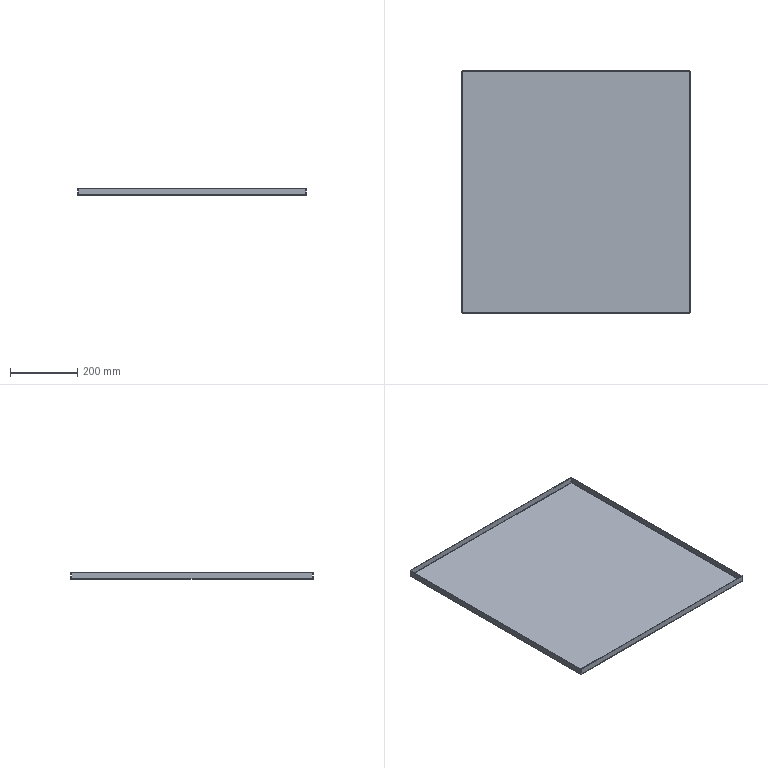Part | STEP file | Part 8 | 1 solid | 38 faces | box 680 x 720 x 20 mm | volume 1075588 mm3 | plane 22 | spline 8 | cylinder 8 | commonest cylinder face diameters 1 x4 5 x4
STEP:
#1=CARTESIAN_POINT('',(-337.5,-357.5,-2.));
#2=VERTEX_POINT('',#1);
#3=CARTESIAN_POINT('',(-337.5,357.5,-2.));
#4=VERTEX_POINT('',#3);
#5=CARTESIAN_POINT('',(-337.5,-357.5,-2.));
#6=DIRECTION('',(0.,1.,0.));
#7=VECTOR('',#6,1000.);
#8=LINE('',#5,#7);
#9=EDGE_CURVE('',#2,#4,#8,.T.);
#10=ORIENTED_EDGE('',*,*,#9,.T.);
#11=CARTESIAN_POINT('',(337.5,357.5,-2.));
#12=VERTEX_POINT('',#11);
#13=CARTESIAN_POINT('',(-337.5,357.5,-2.));
#14=DIRECTION('',(1.,0.,0.));
#15=VECTOR('',#14,1000.);
#16=LINE('',#13,#15);
#17=EDGE_CURVE('',#4,#12,#16,.T.);
#18=ORIENTED_EDGE('',*,*,#17,.T.);
#19=CARTESIAN_POINT('',(337.5,-357.5,-2.));
#20=VERTEX_POINT('',#19);
#21=CARTESIAN_POINT('',(337.5,357.5,-2.));
#22=DIRECTION('',(0.,-1.,0.));
#23=VECTOR('',#22,1000.);
#24=LINE('',#21,#23);
#25=EDGE_CURVE('',#12,#20,#24,.T.);
#26=ORIENTED_EDGE('',*,*,#25,.T.);
#27=CARTESIAN_POINT('',(337.5,-357.5,-2.));
#28=DIRECTION('',(-1.,0.,0.));
#29=VECTOR('',#28,1000.);
#30=LINE('',#27,#29);
#31=EDGE_CURVE('',#20,#2,#30,.T.);
#32=ORIENTED_EDGE('',*,*,#31,.T.);
#33=EDGE_LOOP('',(#10,#18,#26,#32));
#34=FACE_OUTER_BOUND('',#33,.T.);
#35=CARTESIAN_POINT('',(0.,0.,-2.));
#36=DIRECTION('',(0.,0.,1.));
#37=DIRECTION('',(1.,0.,0.));
#38=AXIS2_PLACEMENT_3D('',#35,#36,#37);
#39=PLANE('',#38);
#40=ADVANCED_FACE('',(#34),#39,.F.);
#41=CARTESIAN_POINT('',(-337.5,357.5,0.));
#42=VERTEX_POINT('',#41);
#43=CARTESIAN_POINT('',(337.5,357.5,0.));
#44=VERTEX_POINT('',#43);
#45=CARTESIAN_POINT('',(-337.5,357.5,0.));
#46=DIRECTION('',(1.,0.,0.));
#47=VECTOR('',#46,1000.);
#48=LINE('',#45,#47);
#49=EDGE_CURVE('',#42,#44,#48,.T.);
#50=ORIENTED_EDGE('',*,*,#49,.F.);
#51=CARTESIAN_POINT('',(-337.5,-357.5,0.));
#52=VERTEX_POINT('',#51);
#53=CARTESIAN_POINT('',(-337.5,-357.5,0.));
#54=DIRECTION('',(0.,1.,0.));
#55=VECTOR('',#54,1000.);
#56=LINE('',#53,#55);
#57=EDGE_CURVE('',#52,#42,#56,.T.);
#58=ORIENTED_EDGE('',*,*,#57,.F.);
#59=CARTESIAN_POINT('',(337.5,-357.5,0.));
#60=VERTEX_POINT('',#59);
#61=CARTESIAN_POINT('',(337.5,-357.5,0.));
#62=DIRECTION('',(-1.,0.,0.));
#63=VECTOR('',#62,1000.);
#64=LINE('',#61,#63);
#65=EDGE_CURVE('',#60,#52,#64,.T.);
#66=ORIENTED_EDGE('',*,*,#65,.F.);
#67=CARTESIAN_POINT('',(337.5,357.5,0.));
#68=DIRECTION('',(0.,-1.,0.));
#69=VECTOR('',#68,1000.);
#70=LINE('',#67,#69);
#71=EDGE_CURVE('',#44,#60,#70,.T.);
#72=ORIENTED_EDGE('',*,*,#71,.F.);
#73=EDGE_LOOP('',(#50,#58,#66,#72));
#74=FACE_OUTER_BOUND('',#73,.T.);
#75=CARTESIAN_POINT('',(0.,0.,0.));
#76=DIRECTION('',(0.,0.,1.));
#77=DIRECTION('',(1.,0.,0.));
#78=AXIS2_PLACEMENT_3D('',#75,#76,#77);
#79=PLANE('',#78);
#80=ADVANCED_FACE('',(#74),#79,.T.);
#81=CARTESIAN_POINT('',(337.293,360.,0.5));
#82=VERTEX_POINT('',#81);
#83=CARTESIAN_POINT('',(337.293,358.,0.5));
#84=VERTEX_POINT('',#83);
#85=CARTESIAN_POINT('',(337.293,358.,0.5));
#86=DIRECTION('',(0.,-1.,0.));
#87=VECTOR('',#86,1000.);
#88=LINE('',#85,#87);
#89=EDGE_CURVE('',#82,#84,#88,.T.);
#90=ORIENTED_EDGE('',*,*,#89,.T.);
#91=CARTESIAN_POINT('',(337.5,357.5,0.));
#92=CARTESIAN_POINT('',(337.465,357.631,0.));
#93=CARTESIAN_POINT('',(337.431,357.761,0.05389));
#94=CARTESIAN_POINT('',(337.362,357.946,0.239));
#95=CARTESIAN_POINT('',(337.327,358.,0.3691));
#96=CARTESIAN_POINT('',(337.293,358.,0.5));
#97=B_SPLINE_CURVE_WITH_KNOTS('',3,(#91,#92,#93,#94,#95,#96),.UNSPECIFIED.,.F.,.F.,(4,2,4),(0.,0.5,1.),.UNSPECIFIED.);
#98=EDGE_CURVE('',#44,#84,#97,.T.);
#99=ORIENTED_EDGE('',*,*,#98,.F.);
#100=CARTESIAN_POINT('',(337.5,357.5,0.));
#101=DIRECTION('',(0.,0.,-1.));
#102=VECTOR('',#101,1000.);
#103=LINE('',#100,#102);
#104=EDGE_CURVE('',#44,#12,#103,.T.);
#105=ORIENTED_EDGE('',*,*,#104,.T.);
#106=CARTESIAN_POINT('',(337.5,357.5,-2.));
#107=CARTESIAN_POINT('',(337.483,357.827,-2.));
#108=CARTESIAN_POINT('',(337.465,358.154,-1.935));
#109=CARTESIAN_POINT('',(337.431,358.759,-1.684));
#110=CARTESIAN_POINT('',(337.414,359.036,-1.499));
#111=CARTESIAN_POINT('',(337.379,359.499,-1.036));
#112=CARTESIAN_POINT('',(337.362,359.684,-0.759));
#113=CARTESIAN_POINT('',(337.327,359.935,-0.1544));
#114=CARTESIAN_POINT('',(337.31,360.,0.1728));
#115=CARTESIAN_POINT('',(337.293,360.,0.5));
#116=B_SPLINE_CURVE_WITH_KNOTS('',3,(#106,#107,#108,#109,#110,#111,#112,#113,#114,#115),.UNSPECIFIED.,.F.,.F.,(4,2,2,2,4),(0.,0.25,0.5,0.75,1.),.UNSPECIFIED.);
#117=EDGE_CURVE('',#12,#82,#116,.T.);
#118=ORIENTED_EDGE('',*,*,#117,.T.);
#119=EDGE_LOOP('',(#90,#99,#105,#118));
#120=FACE_OUTER_BOUND('',#119,.T.);
#121=CARTESIAN_POINT('',(337.5,357.5,-2.02));
#122=CARTESIAN_POINT('',(337.483,357.83,-2.02));
#123=CARTESIAN_POINT('',(337.465,358.16,-1.954));
#124=CARTESIAN_POINT('',(337.431,358.769,-1.702));
#125=CARTESIAN_POINT('',(337.414,359.049,-1.515));
#126=CARTESIAN_POINT('',(337.379,359.515,-1.049));
#127=CARTESIAN_POINT('',(337.362,359.702,-0.7691));
#128=CARTESIAN_POINT('',(337.327,359.954,-0.1596));
#129=CARTESIAN_POINT('',(337.31,360.02,0.1701));
#130=CARTESIAN_POINT('',(337.293,360.02,0.5));
#131=CARTESIAN_POINT('',(337.5,357.5,-2.));
#132=CARTESIAN_POINT('',(337.483,357.827,-2.));
#133=CARTESIAN_POINT('',(337.465,358.154,-1.935));
#134=CARTESIAN_POINT('',(337.431,358.759,-1.684));
#135=CARTESIAN_POINT('',(337.414,359.036,-1.499));
#136=CARTESIAN_POINT('',(337.379,359.499,-1.036));
#137=CARTESIAN_POINT('',(337.362,359.684,-0.759));
#138=CARTESIAN_POINT('',(337.327,359.935,-0.1544));
#139=CARTESIAN_POINT('',(337.31,360.,0.1727));
#140=CARTESIAN_POINT('',(337.293,360.,0.5));
#141=CARTESIAN_POINT('',(337.5,357.5,0.));
#142=CARTESIAN_POINT('',(337.483,357.565,0.));
#143=CARTESIAN_POINT('',(337.465,357.631,0.01301));
#144=CARTESIAN_POINT('',(337.431,357.752,0.06311));
#145=CARTESIAN_POINT('',(337.414,357.807,0.1002));
#146=CARTESIAN_POINT('',(337.379,357.9,0.1927));
#147=CARTESIAN_POINT('',(337.362,357.937,0.2482));
#148=CARTESIAN_POINT('',(337.327,357.987,0.3691));
#149=CARTESIAN_POINT('',(337.31,358.,0.4345));
#150=CARTESIAN_POINT('',(337.293,358.,0.5));
#151=CARTESIAN_POINT('',(337.5,357.5,0.0202));
#152=CARTESIAN_POINT('',(337.483,357.563,0.0202));
#153=CARTESIAN_POINT('',(337.465,357.626,0.03269));
#154=CARTESIAN_POINT('',(337.431,357.742,0.08076));
#155=CARTESIAN_POINT('',(337.414,357.795,0.1163));
#156=CARTESIAN_POINT('',(337.379,357.884,0.2051));
#157=CARTESIAN_POINT('',(337.362,357.919,0.2584));
#158=CARTESIAN_POINT('',(337.327,357.967,0.3744));
#159=CARTESIAN_POINT('',(337.31,357.98,0.4372));
#160=CARTESIAN_POINT('',(337.293,357.98,0.5));
#161=B_SPLINE_SURFACE_WITH_KNOTS('',1,3,((#121,#122,#123,#124,#125,#126,#127,#128,#129,#130),(#131,#132,#133,#134,#135,#136,#137,#138,#139,#140),(#141,#142,#143,#144,#145,#146,#147,#148,#149,#150),(#151,#152,#153,#154,#155,#156,#157,#158,#159,#160)),.UNSPECIFIED.,.F.,.F.,.F.,(2,1,1,2),(4,2,2,2,4),(-0.01,0.,1.,1.01),(0.,0.25,0.5,0.75,1.),.UNSPECIFIED.);
#162=ADVANCED_FACE('',(#120),#161,.F.);
#163=CARTESIAN_POINT('',(-337.293,358.,0.5));
#164=VERTEX_POINT('',#163);
#165=CARTESIAN_POINT('',(-337.293,358.,0.5));
#166=CARTESIAN_POINT('',(-337.327,358.,0.3691));
#167=CARTESIAN_POINT('',(-337.362,357.946,0.239));
#168=CARTESIAN_POINT('',(-337.431,357.761,0.05389));
#169=CARTESIAN_POINT('',(-337.465,357.631,0.));
#170=CARTESIAN_POINT('',(-337.5,357.5,0.));
#171=B_SPLINE_CURVE_WITH_KNOTS('',3,(#165,#166,#167,#168,#169,#170),.UNSPECIFIED.,.F.,.F.,(4,2,4),(0.,0.5,1.),.UNSPECIFIED.);
#172=EDGE_CURVE('',#164,#42,#171,.T.);
#173=ORIENTED_EDGE('',*,*,#172,.F.);
#174=CARTESIAN_POINT('',(-337.293,360.,0.5));
#175=VERTEX_POINT('',#174);
#176=CARTESIAN_POINT('',(-337.293,358.,0.5));
#177=DIRECTION('',(0.,-1.,0.));
#178=VECTOR('',#177,1000.);
#179=LINE('',#176,#178);
#180=EDGE_CURVE('',#175,#164,#179,.T.);
#181=ORIENTED_EDGE('',*,*,#180,.F.);
#182=CARTESIAN_POINT('',(-337.293,360.,0.5));
#183=CARTESIAN_POINT('',(-337.31,360.,0.1728));
#184=CARTESIAN_POINT('',(-337.327,359.935,-0.1544));
#185=CARTESIAN_POINT('',(-337.362,359.684,-0.759));
#186=CARTESIAN_POINT('',(-337.379,359.499,-1.036));
#187=CARTESIAN_POINT('',(-337.414,359.036,-1.499));
#188=CARTESIAN_POINT('',(-337.431,358.759,-1.684));
#189=CARTESIAN_POINT('',(-337.465,358.154,-1.935));
#190=CARTESIAN_POINT('',(-337.483,357.827,-2.));
#191=CARTESIAN_POINT('',(-337.5,357.5,-2.));
#192=B_SPLINE_CURVE_WITH_KNOTS('',3,(#182,#183,#184,#185,#186,#187,#188,#189,#190,#191),.UNSPECIFIED.,.F.,.F.,(4,2,2,2,4),(0.,0.25,0.5,0.75,1.),.UNSPECIFIED.);
#193=EDGE_CURVE('',#175,#4,#192,.T.);
#194=ORIENTED_EDGE('',*,*,#193,.T.);
#195=CARTESIAN_POINT('',(-337.5,357.5,0.));
#196=DIRECTION('',(0.,0.,-1.));
#197=VECTOR('',#196,1000.);
#198=LINE('',#195,#197);
#199=EDGE_CURVE('',#42,#4,#198,.T.);
#200=ORIENTED_EDGE('',*,*,#199,.F.);
#201=EDGE_LOOP('',(#173,#181,#194,#200));
#202=FACE_OUTER_BOUND('',#201,.T.);
#203=CARTESIAN_POINT('',(-337.293,360.02,0.5));
#204=CARTESIAN_POINT('',(-337.31,360.02,0.1701));
#205=CARTESIAN_POINT('',(-337.327,359.954,-0.1596));
#206=CARTESIAN_POINT('',(-337.362,359.702,-0.7691));
#207=CARTESIAN_POINT('',(-337.379,359.515,-1.049));
#208=CARTESIAN_POINT('',(-337.414,359.049,-1.515));
#209=CARTESIAN_POINT('',(-337.431,358.769,-1.702));
#210=CARTESIAN_POINT('',(-337.465,358.16,-1.954));
#211=CARTESIAN_POINT('',(-337.483,357.83,-2.02));
#212=CARTESIAN_POINT('',(-337.5,357.5,-2.02));
#213=CARTESIAN_POINT('',(-337.293,360.,0.5));
#214=CARTESIAN_POINT('',(-337.31,360.,0.1727));
#215=CARTESIAN_POINT('',(-337.327,359.935,-0.1544));
#216=CARTESIAN_POINT('',(-337.362,359.684,-0.759));
#217=CARTESIAN_POINT('',(-337.379,359.499,-1.036));
#218=CARTESIAN_POINT('',(-337.414,359.036,-1.499));
#219=CARTESIAN_POINT('',(-337.431,358.759,-1.684));
#220=CARTESIAN_POINT('',(-337.465,358.154,-1.935));
#221=CARTESIAN_POINT('',(-337.483,357.827,-2.));
#222=CARTESIAN_POINT('',(-337.5,357.5,-2.));
#223=CARTESIAN_POINT('',(-337.293,358.,0.5));
#224=CARTESIAN_POINT('',(-337.31,358.,0.4345));
#225=CARTESIAN_POINT('',(-337.327,357.987,0.3691));
#226=CARTESIAN_POINT('',(-337.362,357.937,0.2482));
#227=CARTESIAN_POINT('',(-337.379,357.9,0.1927));
#228=CARTESIAN_POINT('',(-337.414,357.807,0.1002));
#229=CARTESIAN_POINT('',(-337.431,357.752,0.06311));
#230=CARTESIAN_POINT('',(-337.465,357.631,0.01301));
#231=CARTESIAN_POINT('',(-337.483,357.565,0.));
#232=CARTESIAN_POINT('',(-337.5,357.5,0.));
#233=CARTESIAN_POINT('',(-337.293,357.98,0.5));
#234=CARTESIAN_POINT('',(-337.31,357.98,0.4372));
#235=CARTESIAN_POINT('',(-337.327,357.967,0.3744));
#236=CARTESIAN_POINT('',(-337.362,357.919,0.2584));
#237=CARTESIAN_POINT('',(-337.379,357.884,0.2051));
#238=CARTESIAN_POINT('',(-337.414,357.795,0.1163));
#239=CARTESIAN_POINT('',(-337.431,357.742,0.08076));
#240=CARTESIAN_POINT('',(-337.465,357.626,0.03269));
#241=CARTESIAN_POINT('',(-337.483,357.563,0.0202));
#242=CARTESIAN_POINT('',(-337.5,357.5,0.0202));
#243=B_SPLINE_SURFACE_WITH_KNOTS('',1,3,((#203,#204,#205,#206,#207,#208,#209,#210,#211,#212),(#213,#214,#215,#216,#217,#218,#219,#220,#221,#222),(#223,#224,#225,#226,#227,#228,#229,#230,#231,#232),(#233,#234,#235,#236,#237,#238,#239,#240,#241,#242)),.UNSPECIFIED.,.F.,.F.,.F.,(2,1,1,2),(4,2,2,2,4),(-0.01,0.,1.,1.01),(0.,0.25,0.5,0.75,1.),.UNSPECIFIED.);
#244=ADVANCED_FACE('',(#202),#243,.F.);
#245=ORIENTED_EDGE('',*,*,#17,.F.);
#246=ORIENTED_EDGE('',*,*,#193,.F.);
#247=CARTESIAN_POINT('',(0.,360.,0.5));
#248=DIRECTION('',(-1.,0.,0.));
#249=VECTOR('',#248,1000.);
#250=LINE('',#247,#249);
#251=EDGE_CURVE('',#82,#175,#250,.T.);
#252=ORIENTED_EDGE('',*,*,#251,.F.);
#253=ORIENTED_EDGE('',*,*,#117,.F.);
#254=EDGE_LOOP('',(#245,#246,#252,#253));
#255=FACE_OUTER_BOUND('',#254,.T.);
#256=CARTESIAN_POINT('',(-337.5,357.5,0.5));
#257=DIRECTION('',(-1.,0.,0.));
#258=DIRECTION('',(0.,1.,0.));
#259=AXIS2_PLACEMENT_3D('',#256,#257,#258);
#260=CYLINDRICAL_SURFACE('',#259,2.5);
#261=ADVANCED_FACE('',(#255),#260,.T.);
#262=ORIENTED_EDGE('',*,*,#49,.T.);
#263=ORIENTED_EDGE('',*,*,#98,.T.);
#264=CARTESIAN_POINT('',(340.,358.,0.5));
#265=DIRECTION('',(-1.,0.,0.));
#266=VECTOR('',#265,1000.);
#267=LINE('',#264,#266);
#268=EDGE_CURVE('',#84,#164,#267,.T.);
#269=ORIENTED_EDGE('',*,*,#268,.T.);
#270=ORIENTED_EDGE('',*,*,#172,.T.);
#271=EDGE_LOOP('',(#262,#263,#269,#270));
#272=FACE_OUTER_BOUND('',#271,.T.);
#273=CARTESIAN_POINT('',(-337.5,357.5,0.5));
#274=DIRECTION('',(-1.,0.,0.));
#275=DIRECTION('',(0.,1.,0.));
#276=AXIS2_PLACEMENT_3D('',#273,#274,#275);
#277=CYLINDRICAL_SURFACE('',#276,0.5);
#278=ADVANCED_FACE('',(#272),#277,.F.);
#279=CARTESIAN_POINT('',(337.293,358.,18.));
#280=VERTEX_POINT('',#279);
#281=CARTESIAN_POINT('',(337.293,360.,18.));
#282=VERTEX_POINT('',#281);
#283=CARTESIAN_POINT('',(337.293,360.,18.));
#284=DIRECTION('',(0.,1.,0.));
#285=VECTOR('',#284,1000.);
#286=LINE('',#283,#285);
#287=EDGE_CURVE('',#280,#282,#286,.T.);
#288=ORIENTED_EDGE('',*,*,#287,.F.);
#289=CARTESIAN_POINT('',(337.293,358.,0.));
#290=DIRECTION('',(0.,0.,1.));
#291=VECTOR('',#290,1000.);
#292=LINE('',#289,#291);
#293=EDGE_CURVE('',#84,#280,#292,.T.);
#294=ORIENTED_EDGE('',*,*,#293,.F.);
#295=ORIENTED_EDGE('',*,*,#89,.F.);
#296=CARTESIAN_POINT('',(337.293,360.,0.));
#297=DIRECTION('',(0.,0.,-1.));
#298=VECTOR('',#297,1000.);
#299=LINE('',#296,#298);
#300=EDGE_CURVE('',#282,#82,#299,.T.);
#301=ORIENTED_EDGE('',*,*,#300,.F.);
#302=EDGE_LOOP('',(#288,#294,#295,#301));
#303=FACE_OUTER_BOUND('',#302,.T.);
#304=CARTESIAN_POINT('',(337.293,358.,0.));
#305=DIRECTION('',(1.,0.,0.));
#306=DIRECTION('',(0.,0.,-1.));
#307=AXIS2_PLACEMENT_3D('',#304,#305,#306);
#308=PLANE('',#307);
#309=ADVANCED_FACE('',(#303),#308,.T.);
#310=CARTESIAN_POINT('',(-337.293,360.,18.));
#311=VERTEX_POINT('',#310);
#312=CARTESIAN_POINT('',(-337.293,360.,0.));
#313=DIRECTION('',(0.,0.,-1.));
#314=VECTOR('',#313,1000.);
#315=LINE('',#312,#314);
#316=EDGE_CURVE('',#311,#175,#315,.T.);
#317=ORIENTED_EDGE('',*,*,#316,.F.);
#318=CARTESIAN_POINT('',(-340.,360.,18.));
#319=DIRECTION('',(-1.,0.,0.));
#320=VECTOR('',#319,1000.);
#321=LINE('',#318,#320);
#322=EDGE_CURVE('',#282,#311,#321,.T.);
#323=ORIENTED_EDGE('',*,*,#322,.F.);
#324=ORIENTED_EDGE('',*,*,#300,.T.);
#325=ORIENTED_EDGE('',*,*,#251,.T.);
#326=EDGE_LOOP('',(#317,#323,#324,#325));
#327=FACE_OUTER_BOUND('',#326,.T.);
#328=CARTESIAN_POINT('',(0.,360.,0.));
#329=DIRECTION('',(0.,1.,0.));
#330=DIRECTION('',(0.,0.,1.));
#331=AXIS2_PLACEMENT_3D('',#328,#329,#330);
#332=PLANE('',#331);
#333=ADVANCED_FACE('',(#327),#332,.T.);
#334=CARTESIAN_POINT('',(-337.293,358.,18.));
#335=VERTEX_POINT('',#334);
#336=CARTESIAN_POINT('',(0.,358.,18.));
#337=DIRECTION('',(-1.,0.,0.));
#338=VECTOR('',#337,1000.);
#339=LINE('',#336,#338);
#340=EDGE_CURVE('',#280,#335,#339,.T.);
#341=ORIENTED_EDGE('',*,*,#340,.T.);
#342=CARTESIAN_POINT('',(-337.293,358.,0.));
#343=DIRECTION('',(0.,0.,1.));
#344=VECTOR('',#343,1000.);
#345=LINE('',#342,#344);
#346=EDGE_CURVE('',#164,#335,#345,.T.);
#347=ORIENTED_EDGE('',*,*,#346,.F.);
#348=ORIENTED_EDGE('',*,*,#268,.F.);
#349=ORIENTED_EDGE('',*,*,#293,.T.);
#350=EDGE_LOOP('',(#341,#347,#348,#349));
#351=FACE_OUTER_BOUND('',#350,.T.);
#352=CARTESIAN_POINT('',(0.,358.,0.));
#353=DIRECTION('',(0.,1.,0.));
#354=DIRECTION('',(0.,0.,1.));
#355=AXIS2_PLACEMENT_3D('',#352,#353,#354);
#356=PLANE('',#355);
#357=ADVANCED_FACE('',(#351),#356,.F.);
#358=CARTESIAN_POINT('',(-337.293,358.,18.));
#359=DIRECTION('',(0.,1.,0.));
#360=VECTOR('',#359,1000.);
#361=LINE('',#358,#360);
#362=EDGE_CURVE('',#335,#311,#361,.T.);
#363=ORIENTED_EDGE('',*,*,#362,.F.);
#364=ORIENTED_EDGE('',*,*,#340,.F.);
#365=ORIENTED_EDGE('',*,*,#287,.T.);
#366=ORIENTED_EDGE('',*,*,#322,.T.);
#367=EDGE_LOOP('',(#363,#364,#365,#366));
#368=FACE_OUTER_BOUND('',#367,.T.);
#369=CARTESIAN_POINT('',(-340.,360.,18.));
#370=DIRECTION('',(0.,0.,1.));
#371=DIRECTION('',(0.,-1.,0.));
#372=AXIS2_PLACEMENT_3D('',#369,#370,#371);
#373=PLANE('',#372);
#374=ADVANCED_FACE('',(#368),#373,.T.);
#375=ORIENTED_EDGE('',*,*,#346,.T.);
#376=ORIENTED_EDGE('',*,*,#362,.T.);
#377=ORIENTED_EDGE('',*,*,#316,.T.);
#378=ORIENTED_EDGE('',*,*,#180,.T.);
#379=EDGE_LOOP('',(#375,#376,#377,#378));
#380=FACE_OUTER_BOUND('',#379,.T.);
#381=CARTESIAN_POINT('',(-337.293,358.,0.));
#382=DIRECTION('',(1.,0.,0.));
#383=DIRECTION('',(0.,0.,-1.));
#384=AXIS2_PLACEMENT_3D('',#381,#382,#383);
#385=PLANE('',#384);
#386=ADVANCED_FACE('',(#380),#385,.F.);
#387=CARTESIAN_POINT('',(340.,-357.293,0.5));
#388=VERTEX_POINT('',#387);
#389=CARTESIAN_POINT('',(338.,-357.293,0.5));
#390=VERTEX_POINT('',#389);
#391=CARTESIAN_POINT('',(338.,-357.293,0.5));
#392=DIRECTION('',(-1.,0.,0.));
#393=VECTOR('',#392,1000.);
#394=LINE('',#391,#393);
#395=EDGE_CURVE('',#388,#390,#394,.T.);
#396=ORIENTED_EDGE('',*,*,#395,.T.);
#397=CARTESIAN_POINT('',(337.5,-357.5,0.));
#398=CARTESIAN_POINT('',(337.631,-357.465,0.));
#399=CARTESIAN_POINT('',(337.761,-357.431,0.05389));
#400=CARTESIAN_POINT('',(337.946,-357.362,0.239));
#401=CARTESIAN_POINT('',(338.,-357.327,0.3691));
#402=CARTESIAN_POINT('',(338.,-357.293,0.5));
#403=B_SPLINE_CURVE_WITH_KNOTS('',3,(#397,#398,#399,#400,#401,#402),.UNSPECIFIED.,.F.,.F.,(4,2,4),(0.,0.5,1.),.UNSPECIFIED.);
#404=EDGE_CURVE('',#60,#390,#403,.T.);
#405=ORIENTED_EDGE('',*,*,#404,.F.);
#406=CARTESIAN_POINT('',(337.5,-357.5,0.));
#407=DIRECTION('',(0.,0.,-1.));
#408=VECTOR('',#407,1000.);
#409=LINE('',#406,#408);
#410=EDGE_CURVE('',#60,#20,#409,.T.);
#411=ORIENTED_EDGE('',*,*,#410,.T.);
#412=CARTESIAN_POINT('',(337.5,-357.5,-2.));
#413=CARTESIAN_POINT('',(337.827,-357.483,-2.));
#414=CARTESIAN_POINT('',(338.154,-357.465,-1.935));
#415=CARTESIAN_POINT('',(338.759,-357.431,-1.684));
#416=CARTESIAN_POINT('',(339.036,-357.414,-1.499));
#417=CARTESIAN_POINT('',(339.499,-357.379,-1.036));
#418=CARTESIAN_POINT('',(339.684,-357.362,-0.759));
#419=CARTESIAN_POINT('',(339.935,-357.327,-0.1544));
#420=CARTESIAN_POINT('',(340.,-357.31,0.1728));
#421=CARTESIAN_POINT('',(340.,-357.293,0.5));
#422=B_SPLINE_CURVE_WITH_KNOTS('',3,(#412,#413,#414,#415,#416,#417,#418,#419,#420,#421),.UNSPECIFIED.,.F.,.F.,(4,2,2,2,4),(0.,0.25,0.5,0.75,1.),.UNSPECIFIED.);
#423=EDGE_CURVE('',#20,#388,#422,.T.);
#424=ORIENTED_EDGE('',*,*,#423,.T.);
#425=EDGE_LOOP('',(#396,#405,#411,#424));
#426=FACE_OUTER_BOUND('',#425,.T.);
#427=CARTESIAN_POINT('',(337.5,-357.5,-2.02));
#428=CARTESIAN_POINT('',(337.83,-357.483,-2.02));
#429=CARTESIAN_POINT('',(338.16,-357.465,-1.954));
#430=CARTESIAN_POINT('',(338.769,-357.431,-1.702));
#431=CARTESIAN_POINT('',(339.049,-357.414,-1.515));
#432=CARTESIAN_POINT('',(339.515,-357.379,-1.049));
#433=CARTESIAN_POINT('',(339.702,-357.362,-0.7691));
#434=CARTESIAN_POINT('',(339.954,-357.327,-0.1596));
#435=CARTESIAN_POINT('',(340.02,-357.31,0.1701));
#436=CARTESIAN_POINT('',(340.02,-357.293,0.5));
#437=CARTESIAN_POINT('',(337.5,-357.5,-2.));
#438=CARTESIAN_POINT('',(337.827,-357.483,-2.));
#439=CARTESIAN_POINT('',(338.154,-357.465,-1.935));
#440=CARTESIAN_POINT('',(338.759,-357.431,-1.684));
#441=CARTESIAN_POINT('',(339.036,-357.414,-1.499));
#442=CARTESIAN_POINT('',(339.499,-357.379,-1.036));
#443=CARTESIAN_POINT('',(339.684,-357.362,-0.759));
#444=CARTESIAN_POINT('',(339.935,-357.327,-0.1544));
#445=CARTESIAN_POINT('',(340.,-357.31,0.1727));
#446=CARTESIAN_POINT('',(340.,-357.293,0.5));
#447=CARTESIAN_POINT('',(337.5,-357.5,0.));
#448=CARTESIAN_POINT('',(337.565,-357.483,0.));
#449=CARTESIAN_POINT('',(337.631,-357.465,0.01301));
#450=CARTESIAN_POINT('',(337.752,-357.431,0.06311));
#451=CARTESIAN_POINT('',(337.807,-357.414,0.1002));
#452=CARTESIAN_POINT('',(337.9,-357.379,0.1927));
#453=CARTESIAN_POINT('',(337.937,-357.362,0.2482));
#454=CARTESIAN_POINT('',(337.987,-357.327,0.3691));
#455=CARTESIAN_POINT('',(338.,-357.31,0.4345));
#456=CARTESIAN_POINT('',(338.,-357.293,0.5));
#457=CARTESIAN_POINT('',(337.5,-357.5,0.0202));
#458=CARTESIAN_POINT('',(337.563,-357.483,0.0202));
#459=CARTESIAN_POINT('',(337.626,-357.465,0.03269));
#460=CARTESIAN_POINT('',(337.742,-357.431,0.08076));
#461=CARTESIAN_POINT('',(337.795,-357.414,0.1163));
#462=CARTESIAN_POINT('',(337.884,-357.379,0.2051));
#463=CARTESIAN_POINT('',(337.919,-357.362,0.2584));
#464=CARTESIAN_POINT('',(337.967,-357.327,0.3744));
#465=CARTESIAN_POINT('',(337.98,-357.31,0.4372));
#466=CARTESIAN_POINT('',(337.98,-357.293,0.5));
#467=B_SPLINE_SURFACE_WITH_KNOTS('',1,3,((#427,#428,#429,#430,#431,#432,#433,#434,#435,#436),(#437,#438,#439,#440,#441,#442,#443,#444,#445,#446),(#447,#448,#449,#450,#451,#452,#453,#454,#455,#456),(#457,#458,#459,#460,#461,#462,#463,#464,#465,#466)),.UNSPECIFIED.,.F.,.F.,.F.,(2,1,1,2),(4,2,2,2,4),(-0.01,0.,1.,1.01),(0.,0.25,0.5,0.75,1.),.UNSPECIFIED.);
#468=ADVANCED_FACE('',(#426),#467,.F.);
#469=CARTESIAN_POINT('',(338.,357.293,0.5));
#470=VERTEX_POINT('',#469);
#471=CARTESIAN_POINT('',(338.,357.293,0.5));
#472=CARTESIAN_POINT('',(338.,357.327,0.3691));
#473=CARTESIAN_POINT('',(337.946,357.362,0.239));
#474=CARTESIAN_POINT('',(337.761,357.431,0.05389));
#475=CARTESIAN_POINT('',(337.631,357.465,0.));
#476=CARTESIAN_POINT('',(337.5,357.5,0.));
#477=B_SPLINE_CURVE_WITH_KNOTS('',3,(#471,#472,#473,#474,#475,#476),.UNSPECIFIED.,.F.,.F.,(4,2,4),(0.,0.5,1.),.UNSPECIFIED.);
#478=EDGE_CURVE('',#470,#44,#477,.T.);
#479=ORIENTED_EDGE('',*,*,#478,.F.);
#480=CARTESIAN_POINT('',(340.,357.293,0.5));
#481=VERTEX_POINT('',#480);
#482=CARTESIAN_POINT('',(338.,357.293,0.5));
#483=DIRECTION('',(-1.,0.,0.));
#484=VECTOR('',#483,1000.);
#485=LINE('',#482,#484);
#486=EDGE_CURVE('',#481,#470,#485,.T.);
#487=ORIENTED_EDGE('',*,*,#486,.F.);
#488=CARTESIAN_POINT('',(340.,357.293,0.5));
#489=CARTESIAN_POINT('',(340.,357.31,0.1728));
#490=CARTESIAN_POINT('',(339.935,357.327,-0.1544));
#491=CARTESIAN_POINT('',(339.684,357.362,-0.759));
#492=CARTESIAN_POINT('',(339.499,357.379,-1.036));
#493=CARTESIAN_POINT('',(339.036,357.414,-1.499));
#494=CARTESIAN_POINT('',(338.759,357.431,-1.684));
#495=CARTESIAN_POINT('',(338.154,357.465,-1.935));
#496=CARTESIAN_POINT('',(337.827,357.483,-2.));
#497=CARTESIAN_POINT('',(337.5,357.5,-2.));
#498=B_SPLINE_CURVE_WITH_KNOTS('',3,(#488,#489,#490,#491,#492,#493,#494,#495,#496,#497),.UNSPECIFIED.,.F.,.F.,(4,2,2,2,4),(0.,0.25,0.5,0.75,1.),.UNSPECIFIED.);
#499=EDGE_CURVE('',#481,#12,#498,.T.);
#500=ORIENTED_EDGE('',*,*,#499,.T.);
#501=ORIENTED_EDGE('',*,*,#104,.F.);
#502=EDGE_LOOP('',(#479,#487,#500,#501));
#503=FACE_OUTER_BOUND('',#502,.T.);
#504=CARTESIAN_POINT('',(340.02,357.293,0.5));
#505=CARTESIAN_POINT('',(340.02,357.31,0.1701));
#506=CARTESIAN_POINT('',(339.954,357.327,-0.1596));
#507=CARTESIAN_POINT('',(339.702,357.362,-0.7691));
#508=CARTESIAN_POINT('',(339.515,357.379,-1.049));
#509=CARTESIAN_POINT('',(339.049,357.414,-1.515));
#510=CARTESIAN_POINT('',(338.769,357.431,-1.702));
#511=CARTESIAN_POINT('',(338.16,357.465,-1.954));
#512=CARTESIAN_POINT('',(337.83,357.483,-2.02));
#513=CARTESIAN_POINT('',(337.5,357.5,-2.02));
#514=CARTESIAN_POINT('',(340.,357.293,0.5));
#515=CARTESIAN_POINT('',(340.,357.31,0.1727));
#516=CARTESIAN_POINT('',(339.935,357.327,-0.1544));
#517=CARTESIAN_POINT('',(339.684,357.362,-0.759));
#518=CARTESIAN_POINT('',(339.499,357.379,-1.036));
#519=CARTESIAN_POINT('',(339.036,357.414,-1.499));
#520=CARTESIAN_POINT('',(338.759,357.431,-1.684));
#521=CARTESIAN_POINT('',(338.154,357.465,-1.935));
#522=CARTESIAN_POINT('',(337.827,357.483,-2.));
#523=CARTESIAN_POINT('',(337.5,357.5,-2.));
#524=CARTESIAN_POINT('',(338.,357.293,0.5));
#525=CARTESIAN_POINT('',(338.,357.31,0.4345));
#526=CARTESIAN_POINT('',(337.987,357.327,0.3691));
#527=CARTESIAN_POINT('',(337.937,357.362,0.2482));
#528=CARTESIAN_POINT('',(337.9,357.379,0.1927));
#529=CARTESIAN_POINT('',(337.807,357.414,0.1002));
#530=CARTESIAN_POINT('',(337.752,357.431,0.06311));
#531=CARTESIAN_POINT('',(337.631,357.465,0.01301));
#532=CARTESIAN_POINT('',(337.565,357.483,0.));
#533=CARTESIAN_POINT('',(337.5,357.5,0.));
#534=CARTESIAN_POINT('',(337.98,357.293,0.5));
#535=CARTESIAN_POINT('',(337.98,357.31,0.4372));
#536=CARTESIAN_POINT('',(337.967,357.327,0.3744));
#537=CARTESIAN_POINT('',(337.919,357.362,0.2584));
#538=CARTESIAN_POINT('',(337.884,357.379,0.2051));
#539=CARTESIAN_POINT('',(337.795,357.414,0.1163));
#540=CARTESIAN_POINT('',(337.742,357.431,0.08076));
#541=CARTESIAN_POINT('',(337.626,357.465,0.03269));
#542=CARTESIAN_POINT('',(337.563,357.483,0.0202));
#543=CARTESIAN_POINT('',(337.5,357.5,0.0202));
#544=B_SPLINE_SURFACE_WITH_KNOTS('',1,3,((#504,#505,#506,#507,#508,#509,#510,#511,#512,#513),(#514,#515,#516,#517,#518,#519,#520,#521,#522,#523),(#524,#525,#526,#527,#528,#529,#530,#531,#532,#533),(#534,#535,#536,#537,#538,#539,#540,#541,#542,#543)),.UNSPECIFIED.,.F.,.F.,.F.,(2,1,1,2),(4,2,2,2,4),(-0.01,0.,1.,1.01),(0.,0.25,0.5,0.75,1.),.UNSPECIFIED.);
#545=ADVANCED_FACE('',(#503),#544,.F.);
#546=ORIENTED_EDGE('',*,*,#25,.F.);
#547=ORIENTED_EDGE('',*,*,#499,.F.);
#548=CARTESIAN_POINT('',(340.,-360.,0.5));
#549=DIRECTION('',(0.,-1.,0.));
#550=VECTOR('',#549,1000.);
#551=LINE('',#548,#550);
#552=EDGE_CURVE('',#481,#388,#551,.T.);
#553=ORIENTED_EDGE('',*,*,#552,.T.);
#554=ORIENTED_EDGE('',*,*,#423,.F.);
#555=EDGE_LOOP('',(#546,#547,#553,#554));
#556=FACE_OUTER_BOUND('',#555,.T.);
#557=CARTESIAN_POINT('',(337.5,357.5,0.5));
#558=DIRECTION('',(0.,1.,0.));
#559=DIRECTION('',(1.,0.,0.));
#560=AXIS2_PLACEMENT_3D('',#557,#558,#559);
#561=CYLINDRICAL_SURFACE('',#560,2.5);
#562=ADVANCED_FACE('',(#556),#561,.T.);
#563=ORIENTED_EDGE('',*,*,#71,.T.);
#564=ORIENTED_EDGE('',*,*,#404,.T.);
#565=CARTESIAN_POINT('',(338.,-360.,0.5));
#566=DIRECTION('',(0.,1.,0.));
#567=VECTOR('',#566,1000.);
#568=LINE('',#565,#567);
#569=EDGE_CURVE('',#390,#470,#568,.T.);
#570=ORIENTED_EDGE('',*,*,#569,.T.);
#571=ORIENTED_EDGE('',*,*,#478,.T.);
#572=EDGE_LOOP('',(#563,#564,#570,#571));
#573=FACE_OUTER_BOUND('',#572,.T.);
#574=CARTESIAN_POINT('',(337.5,357.5,0.5));
#575=DIRECTION('',(0.,1.,0.));
#576=DIRECTION('',(1.,0.,0.));
#577=AXIS2_PLACEMENT_3D('',#574,#575,#576);
#578=CYLINDRICAL_SURFACE('',#577,0.5);
#579=ADVANCED_FACE('',(#573),#578,.F.);
#580=CARTESIAN_POINT('',(338.,-357.293,18.));
#581=VERTEX_POINT('',#580);
#582=CARTESIAN_POINT('',(340.,-357.293,18.));
#583=VERTEX_POINT('',#582);
#584=CARTESIAN_POINT('',(340.,-357.293,18.));
#585=DIRECTION('',(1.,0.,0.));
#586=VECTOR('',#585,1000.);
#587=LINE('',#584,#586);
#588=EDGE_CURVE('',#581,#583,#587,.T.);
#589=ORIENTED_EDGE('',*,*,#588,.F.);
#590=CARTESIAN_POINT('',(338.,-357.293,0.));
#591=DIRECTION('',(0.,0.,1.));
#592=VECTOR('',#591,1000.);
#593=LINE('',#590,#592);
#594=EDGE_CURVE('',#390,#581,#593,.T.);
#595=ORIENTED_EDGE('',*,*,#594,.F.);
#596=ORIENTED_EDGE('',*,*,#395,.F.);
#597=CARTESIAN_POINT('',(340.,-357.293,0.));
#598=DIRECTION('',(0.,0.,1.));
#599=VECTOR('',#598,1000.);
#600=LINE('',#597,#599);
#601=EDGE_CURVE('',#388,#583,#600,.T.);
#602=ORIENTED_EDGE('',*,*,#601,.T.);
#603=EDGE_LOOP('',(#589,#595,#596,#602));
#604=FACE_OUTER_BOUND('',#603,.T.);
#605=CARTESIAN_POINT('',(338.,-357.293,0.));
#606=DIRECTION('',(0.,-1.,0.));
#607=DIRECTION('',(0.,0.,-1.));
#608=AXIS2_PLACEMENT_3D('',#605,#606,#607);
#609=PLANE('',#608);
#610=ADVANCED_FACE('',(#604),#609,.T.);
#611=ORIENTED_EDGE('',*,*,#552,.F.);
#612=CARTESIAN_POINT('',(340.,357.293,18.));
#613=VERTEX_POINT('',#612);
#614=CARTESIAN_POINT('',(340.,357.293,0.));
#615=DIRECTION('',(0.,0.,1.));
#616=VECTOR('',#615,1000.);
#617=LINE('',#614,#616);
#618=EDGE_CURVE('',#481,#613,#617,.T.);
#619=ORIENTED_EDGE('',*,*,#618,.T.);
#620=CARTESIAN_POINT('',(340.,-360.,18.));
#621=DIRECTION('',(0.,1.,0.));
#622=VECTOR('',#621,1000.);
#623=LINE('',#620,#622);
#624=EDGE_CURVE('',#583,#613,#623,.T.);
#625=ORIENTED_EDGE('',*,*,#624,.F.);
#626=ORIENTED_EDGE('',*,*,#601,.F.);
#627=EDGE_LOOP('',(#611,#619,#625,#626));
#628=FACE_OUTER_BOUND('',#627,.T.);
#629=CARTESIAN_POINT('',(340.,0.,0.));
#630=DIRECTION('',(-1.,0.,0.));
#631=DIRECTION('',(0.,0.,1.));
#632=AXIS2_PLACEMENT_3D('',#629,#630,#631);
#633=PLANE('',#632);
#634=ADVANCED_FACE('',(#628),#633,.F.);
#635=CARTESIAN_POINT('',(338.,357.293,18.));
#636=VERTEX_POINT('',#635);
#637=CARTESIAN_POINT('',(338.,357.293,0.));
#638=DIRECTION('',(0.,0.,1.));
#639=VECTOR('',#638,1000.);
#640=LINE('',#637,#639);
#641=EDGE_CURVE('',#470,#636,#640,.T.);
#642=ORIENTED_EDGE('',*,*,#641,.F.);
#643=ORIENTED_EDGE('',*,*,#569,.F.);
#644=ORIENTED_EDGE('',*,*,#594,.T.);
#645=CARTESIAN_POINT('',(338.,0.,18.));
#646=DIRECTION('',(0.,1.,0.));
#647=VECTOR('',#646,1000.);
#648=LINE('',#645,#647);
#649=EDGE_CURVE('',#581,#636,#648,.T.);
#650=ORIENTED_EDGE('',*,*,#649,.T.);
#651=EDGE_LOOP('',(#642,#643,#644,#650));
#652=FACE_OUTER_BOUND('',#651,.T.);
#653=CARTESIAN_POINT('',(338.,0.,0.));
#654=DIRECTION('',(-1.,0.,0.));
#655=DIRECTION('',(0.,0.,1.));
#656=AXIS2_PLACEMENT_3D('',#653,#654,#655);
#657=PLANE('',#656);
#658=ADVANCED_FACE('',(#652),#657,.T.);
#659=CARTESIAN_POINT('',(338.,357.293,18.));
#660=DIRECTION('',(1.,0.,0.));
#661=VECTOR('',#660,1000.);
#662=LINE('',#659,#661);
#663=EDGE_CURVE('',#636,#613,#662,.T.);
#664=ORIENTED_EDGE('',*,*,#663,.F.);
#665=ORIENTED_EDGE('',*,*,#649,.F.);
#666=ORIENTED_EDGE('',*,*,#588,.T.);
#667=ORIENTED_EDGE('',*,*,#624,.T.);
#668=EDGE_LOOP('',(#664,#665,#666,#667));
#669=FACE_OUTER_BOUND('',#668,.T.);
#670=CARTESIAN_POINT('',(340.,-360.,18.));
#671=DIRECTION('',(0.,0.,1.));
#672=DIRECTION('',(1.,0.,0.));
#673=AXIS2_PLACEMENT_3D('',#670,#671,#672);
#674=PLANE('',#673);
#675=ADVANCED_FACE('',(#669),#674,.T.);
#676=ORIENTED_EDGE('',*,*,#641,.T.);
#677=ORIENTED_EDGE('',*,*,#663,.T.);
#678=ORIENTED_EDGE('',*,*,#618,.F.);
#679=ORIENTED_EDGE('',*,*,#486,.T.);
#680=EDGE_LOOP('',(#676,#677,#678,#679));
#681=FACE_OUTER_BOUND('',#680,.T.);
#682=CARTESIAN_POINT('',(338.,357.293,0.));
#683=DIRECTION('',(0.,-1.,0.));
#684=DIRECTION('',(0.,0.,-1.));
#685=AXIS2_PLACEMENT_3D('',#682,#683,#684);
#686=PLANE('',#685);
#687=ADVANCED_FACE('',(#681),#686,.F.);
#688=CARTESIAN_POINT('',(-337.293,-360.,0.5));
#689=VERTEX_POINT('',#688);
#690=CARTESIAN_POINT('',(-337.293,-358.,0.5));
#691=VERTEX_POINT('',#690);
#692=CARTESIAN_POINT('',(-337.293,-358.,0.5));
#693=DIRECTION('',(0.,1.,0.));
#694=VECTOR('',#693,1000.);
#695=LINE('',#692,#694);
#696=EDGE_CURVE('',#689,#691,#695,.T.);
#697=ORIENTED_EDGE('',*,*,#696,.T.);
#698=CARTESIAN_POINT('',(-337.5,-357.5,0.));
#699=CARTESIAN_POINT('',(-337.465,-357.631,0.));
#700=CARTESIAN_POINT('',(-337.431,-357.761,0.05389));
#701=CARTESIAN_POINT('',(-337.362,-357.946,0.239));
#702=CARTESIAN_POINT('',(-337.327,-358.,0.3691));
#703=CARTESIAN_POINT('',(-337.293,-358.,0.5));
#704=B_SPLINE_CURVE_WITH_KNOTS('',3,(#698,#699,#700,#701,#702,#703),.UNSPECIFIED.,.F.,.F.,(4,2,4),(0.,0.5,1.),.UNSPECIFIED.);
#705=EDGE_CURVE('',#52,#691,#704,.T.);
#706=ORIENTED_EDGE('',*,*,#705,.F.);
#707=CARTESIAN_POINT('',(-337.5,-357.5,0.));
#708=DIRECTION('',(0.,0.,-1.));
#709=VECTOR('',#708,1000.);
#710=LINE('',#707,#709);
#711=EDGE_CURVE('',#52,#2,#710,.T.);
#712=ORIENTED_EDGE('',*,*,#711,.T.);
#713=CARTESIAN_POINT('',(-337.5,-357.5,-2.));
#714=CARTESIAN_POINT('',(-337.483,-357.827,-2.));
#715=CARTESIAN_POINT('',(-337.465,-358.154,-1.935));
#716=CARTESIAN_POINT('',(-337.431,-358.759,-1.684));
#717=CARTESIAN_POINT('',(-337.414,-359.036,-1.499));
#718=CARTESIAN_POINT('',(-337.379,-359.499,-1.036));
#719=CARTESIAN_POINT('',(-337.362,-359.684,-0.759));
#720=CARTESIAN_POINT('',(-337.327,-359.935,-0.1544));
#721=CARTESIAN_POINT('',(-337.31,-360.,0.1728));
#722=CARTESIAN_POINT('',(-337.293,-360.,0.5));
#723=B_SPLINE_CURVE_WITH_KNOTS('',3,(#713,#714,#715,#716,#717,#718,#719,#720,#721,#722),.UNSPECIFIED.,.F.,.F.,(4,2,2,2,4),(0.,0.25,0.5,0.75,1.),.UNSPECIFIED.);
#724=EDGE_CURVE('',#2,#689,#723,.T.);
#725=ORIENTED_EDGE('',*,*,#724,.T.);
#726=EDGE_LOOP('',(#697,#706,#712,#725));
#727=FACE_OUTER_BOUND('',#726,.T.);
#728=CARTESIAN_POINT('',(-337.5,-357.5,-2.02));
#729=CARTESIAN_POINT('',(-337.483,-357.83,-2.02));
#730=CARTESIAN_POINT('',(-337.465,-358.16,-1.954));
#731=CARTESIAN_POINT('',(-337.431,-358.769,-1.702));
#732=CARTESIAN_POINT('',(-337.414,-359.049,-1.515));
#733=CARTESIAN_POINT('',(-337.379,-359.515,-1.049));
#734=CARTESIAN_POINT('',(-337.362,-359.702,-0.7691));
#735=CARTESIAN_POINT('',(-337.327,-359.954,-0.1596));
#736=CARTESIAN_POINT('',(-337.31,-360.02,0.1701));
#737=CARTESIAN_POINT('',(-337.293,-360.02,0.5));
#738=CARTESIAN_POINT('',(-337.5,-357.5,-2.));
#739=CARTESIAN_POINT('',(-337.483,-357.827,-2.));
#740=CARTESIAN_POINT('',(-337.465,-358.154,-1.935));
#741=CARTESIAN_POINT('',(-337.431,-358.759,-1.684));
#742=CARTESIAN_POINT('',(-337.414,-359.036,-1.499));
#743=CARTESIAN_POINT('',(-337.379,-359.499,-1.036));
#744=CARTESIAN_POINT('',(-337.362,-359.684,-0.759));
#745=CARTESIAN_POINT('',(-337.327,-359.935,-0.1544));
#746=CARTESIAN_POINT('',(-337.31,-360.,0.1727));
#747=CARTESIAN_POINT('',(-337.293,-360.,0.5));
#748=CARTESIAN_POINT('',(-337.5,-357.5,0.));
#749=CARTESIAN_POINT('',(-337.483,-357.565,0.));
#750=CARTESIAN_POINT('',(-337.465,-357.631,0.01301));
#751=CARTESIAN_POINT('',(-337.431,-357.752,0.06311));
#752=CARTESIAN_POINT('',(-337.414,-357.807,0.1002));
#753=CARTESIAN_POINT('',(-337.379,-357.9,0.1927));
#754=CARTESIAN_POINT('',(-337.362,-357.937,0.2482));
#755=CARTESIAN_POINT('',(-337.327,-357.987,0.3691));
#756=CARTESIAN_POINT('',(-337.31,-358.,0.4345));
#757=CARTESIAN_POINT('',(-337.293,-358.,0.5));
#758=CARTESIAN_POINT('',(-337.5,-357.5,0.0202));
#759=CARTESIAN_POINT('',(-337.483,-357.563,0.0202));
#760=CARTESIAN_POINT('',(-337.465,-357.626,0.03269));
#761=CARTESIAN_POINT('',(-337.431,-357.742,0.08076));
#762=CARTESIAN_POINT('',(-337.414,-357.795,0.1163));
#763=CARTESIAN_POINT('',(-337.379,-357.884,0.2051));
#764=CARTESIAN_POINT('',(-337.362,-357.919,0.2584));
#765=CARTESIAN_POINT('',(-337.327,-357.967,0.3744));
#766=CARTESIAN_POINT('',(-337.31,-357.98,0.4372));
#767=CARTESIAN_POINT('',(-337.293,-357.98,0.5));
#768=B_SPLINE_SURFACE_WITH_KNOTS('',1,3,((#728,#729,#730,#731,#732,#733,#734,#735,#736,#737),(#738,#739,#740,#741,#742,#743,#744,#745,#746,#747),(#748,#749,#750,#751,#752,#753,#754,#755,#756,#757),(#758,#759,#760,#761,#762,#763,#764,#765,#766,#767)),.UNSPECIFIED.,.F.,.F.,.F.,(2,1,1,2),(4,2,2,2,4),(-0.01,0.,1.,1.01),(0.,0.25,0.5,0.75,1.),.UNSPECIFIED.);
#769=ADVANCED_FACE('',(#727),#768,.F.);
#770=CARTESIAN_POINT('',(337.293,-358.,0.5));
#771=VERTEX_POINT('',#770);
#772=CARTESIAN_POINT('',(337.293,-358.,0.5));
#773=CARTESIAN_POINT('',(337.327,-358.,0.3691));
#774=CARTESIAN_POINT('',(337.362,-357.946,0.239));
#775=CARTESIAN_POINT('',(337.431,-357.761,0.05389));
#776=CARTESIAN_POINT('',(337.465,-357.631,0.));
#777=CARTESIAN_POINT('',(337.5,-357.5,0.));
#778=B_SPLINE_CURVE_WITH_KNOTS('',3,(#772,#773,#774,#775,#776,#777),.UNSPECIFIED.,.F.,.F.,(4,2,4),(0.,0.5,1.),.UNSPECIFIED.);
#779=EDGE_CURVE('',#771,#60,#778,.T.);
#780=ORIENTED_EDGE('',*,*,#779,.F.);
#781=CARTESIAN_POINT('',(337.293,-360.,0.5));
#782=VERTEX_POINT('',#781);
#783=CARTESIAN_POINT('',(337.293,-358.,0.5));
#784=DIRECTION('',(0.,1.,0.));
#785=VECTOR('',#784,1000.);
#786=LINE('',#783,#785);
#787=EDGE_CURVE('',#782,#771,#786,.T.);
#788=ORIENTED_EDGE('',*,*,#787,.F.);
#789=CARTESIAN_POINT('',(337.293,-360.,0.5));
#790=CARTESIAN_POINT('',(337.31,-360.,0.1728));
#791=CARTESIAN_POINT('',(337.327,-359.935,-0.1544));
#792=CARTESIAN_POINT('',(337.362,-359.684,-0.759));
#793=CARTESIAN_POINT('',(337.379,-359.499,-1.036));
#794=CARTESIAN_POINT('',(337.414,-359.036,-1.499));
#795=CARTESIAN_POINT('',(337.431,-358.759,-1.684));
#796=CARTESIAN_POINT('',(337.465,-358.154,-1.935));
#797=CARTESIAN_POINT('',(337.483,-357.827,-2.));
#798=CARTESIAN_POINT('',(337.5,-357.5,-2.));
#799=B_SPLINE_CURVE_WITH_KNOTS('',3,(#789,#790,#791,#792,#793,#794,#795,#796,#797,#798),.UNSPECIFIED.,.F.,.F.,(4,2,2,2,4),(0.,0.25,0.5,0.75,1.),.UNSPECIFIED.);
#800=EDGE_CURVE('',#782,#20,#799,.T.);
#801=ORIENTED_EDGE('',*,*,#800,.T.);
#802=ORIENTED_EDGE('',*,*,#410,.F.);
#803=EDGE_LOOP('',(#780,#788,#801,#802));
#804=FACE_OUTER_BOUND('',#803,.T.);
#805=CARTESIAN_POINT('',(337.293,-360.02,0.5));
#806=CARTESIAN_POINT('',(337.31,-360.02,0.1701));
#807=CARTESIAN_POINT('',(337.327,-359.954,-0.1596));
#808=CARTESIAN_POINT('',(337.362,-359.702,-0.7691));
#809=CARTESIAN_POINT('',(337.379,-359.515,-1.049));
#810=CARTESIAN_POINT('',(337.414,-359.049,-1.515));
#811=CARTESIAN_POINT('',(337.431,-358.769,-1.702));
#812=CARTESIAN_POINT('',(337.465,-358.16,-1.954));
#813=CARTESIAN_POINT('',(337.483,-357.83,-2.02));
#814=CARTESIAN_POINT('',(337.5,-357.5,-2.02));
#815=CARTESIAN_POINT('',(337.293,-360.,0.5));
#816=CARTESIAN_POINT('',(337.31,-360.,0.1727));
#817=CARTESIAN_POINT('',(337.327,-359.935,-0.1544));
#818=CARTESIAN_POINT('',(337.362,-359.684,-0.759));
#819=CARTESIAN_POINT('',(337.379,-359.499,-1.036));
#820=CARTESIAN_POINT('',(337.414,-359.036,-1.499));
#821=CARTESIAN_POINT('',(337.431,-358.759,-1.684));
#822=CARTESIAN_POINT('',(337.465,-358.154,-1.935));
#823=CARTESIAN_POINT('',(337.483,-357.827,-2.));
#824=CARTESIAN_POINT('',(337.5,-357.5,-2.));
#825=CARTESIAN_POINT('',(337.293,-358.,0.5));
#826=CARTESIAN_POINT('',(337.31,-358.,0.4345));
#827=CARTESIAN_POINT('',(337.327,-357.987,0.3691));
#828=CARTESIAN_POINT('',(337.362,-357.937,0.2482));
#829=CARTESIAN_POINT('',(337.379,-357.9,0.1927));
#830=CARTESIAN_POINT('',(337.414,-357.807,0.1002));
#831=CARTESIAN_POINT('',(337.431,-357.752,0.06311));
#832=CARTESIAN_POINT('',(337.465,-357.631,0.01301));
#833=CARTESIAN_POINT('',(337.483,-357.565,0.));
#834=CARTESIAN_POINT('',(337.5,-357.5,0.));
#835=CARTESIAN_POINT('',(337.293,-357.98,0.5));
#836=CARTESIAN_POINT('',(337.31,-357.98,0.4372));
#837=CARTESIAN_POINT('',(337.327,-357.967,0.3744));
#838=CARTESIAN_POINT('',(337.362,-357.919,0.2584));
#839=CARTESIAN_POINT('',(337.379,-357.884,0.2051));
#840=CARTESIAN_POINT('',(337.414,-357.795,0.1163));
#841=CARTESIAN_POINT('',(337.431,-357.742,0.08076));
#842=CARTESIAN_POINT('',(337.465,-357.626,0.03269));
#843=CARTESIAN_POINT('',(337.483,-357.563,0.0202));
#844=CARTESIAN_POINT('',(337.5,-357.5,0.0202));
#845=B_SPLINE_SURFACE_WITH_KNOTS('',1,3,((#805,#806,#807,#808,#809,#810,#811,#812,#813,#814),(#815,#816,#817,#818,#819,#820,#821,#822,#823,#824),(#825,#826,#827,#828,#829,#830,#831,#832,#833,#834),(#835,#836,#837,#838,#839,#840,#841,#842,#843,#844)),.UNSPECIFIED.,.F.,.F.,.F.,(2,1,1,2),(4,2,2,2,4),(-0.01,0.,1.,1.01),(0.,0.25,0.5,0.75,1.),.UNSPECIFIED.);
#846=ADVANCED_FACE('',(#804),#845,.F.);
#847=ORIENTED_EDGE('',*,*,#31,.F.);
#848=ORIENTED_EDGE('',*,*,#800,.F.);
#849=CARTESIAN_POINT('',(-340.,-360.,0.5));
#850=DIRECTION('',(-1.,0.,0.));
#851=VECTOR('',#850,1000.);
#852=LINE('',#849,#851);
#853=EDGE_CURVE('',#782,#689,#852,.T.);
#854=ORIENTED_EDGE('',*,*,#853,.T.);
#855=ORIENTED_EDGE('',*,*,#724,.F.);
#856=EDGE_LOOP('',(#847,#848,#854,#855));
#857=FACE_OUTER_BOUND('',#856,.T.);
#858=CARTESIAN_POINT('',(337.5,-357.5,0.5));
#859=DIRECTION('',(1.,0.,0.));
#860=DIRECTION('',(0.,-1.,0.));
#861=AXIS2_PLACEMENT_3D('',#858,#859,#860);
#862=CYLINDRICAL_SURFACE('',#861,2.5);
#863=ADVANCED_FACE('',(#857),#862,.T.);
#864=ORIENTED_EDGE('',*,*,#65,.T.);
#865=ORIENTED_EDGE('',*,*,#705,.T.);
#866=CARTESIAN_POINT('',(-340.,-358.,0.5));
#867=DIRECTION('',(1.,0.,0.));
#868=VECTOR('',#867,1000.);
#869=LINE('',#866,#868);
#870=EDGE_CURVE('',#691,#771,#869,.T.);
#871=ORIENTED_EDGE('',*,*,#870,.T.);
#872=ORIENTED_EDGE('',*,*,#779,.T.);
#873=EDGE_LOOP('',(#864,#865,#871,#872));
#874=FACE_OUTER_BOUND('',#873,.T.);
#875=CARTESIAN_POINT('',(337.5,-357.5,0.5));
#876=DIRECTION('',(1.,0.,0.));
#877=DIRECTION('',(0.,-1.,0.));
#878=AXIS2_PLACEMENT_3D('',#875,#876,#877);
#879=CYLINDRICAL_SURFACE('',#878,0.5);
#880=ADVANCED_FACE('',(#874),#879,.F.);
#881=CARTESIAN_POINT('',(-337.293,-358.,18.));
#882=VERTEX_POINT('',#881);
#883=CARTESIAN_POINT('',(-337.293,-360.,18.));
#884=VERTEX_POINT('',#883);
#885=CARTESIAN_POINT('',(-337.293,-360.,18.));
#886=DIRECTION('',(0.,-1.,0.));
#887=VECTOR('',#886,1000.);
#888=LINE('',#885,#887);
#889=EDGE_CURVE('',#882,#884,#888,.T.);
#890=ORIENTED_EDGE('',*,*,#889,.F.);
#891=CARTESIAN_POINT('',(-337.293,-358.,0.));
#892=DIRECTION('',(0.,0.,1.));
#893=VECTOR('',#892,1000.);
#894=LINE('',#891,#893);
#895=EDGE_CURVE('',#691,#882,#894,.T.);
#896=ORIENTED_EDGE('',*,*,#895,.F.);
#897=ORIENTED_EDGE('',*,*,#696,.F.);
#898=CARTESIAN_POINT('',(-337.293,-360.,0.));
#899=DIRECTION('',(0.,0.,1.));
#900=VECTOR('',#899,1000.);
#901=LINE('',#898,#900);
#902=EDGE_CURVE('',#689,#884,#901,.T.);
#903=ORIENTED_EDGE('',*,*,#902,.T.);
#904=EDGE_LOOP('',(#890,#896,#897,#903));
#905=FACE_OUTER_BOUND('',#904,.T.);
#906=CARTESIAN_POINT('',(-337.293,-358.,0.));
#907=DIRECTION('',(-1.,0.,0.));
#908=DIRECTION('',(0.,0.,1.));
#909=AXIS2_PLACEMENT_3D('',#906,#907,#908);
#910=PLANE('',#909);
#911=ADVANCED_FACE('',(#905),#910,.T.);
#912=ORIENTED_EDGE('',*,*,#853,.F.);
#913=CARTESIAN_POINT('',(337.293,-360.,18.));
#914=VERTEX_POINT('',#913);
#915=CARTESIAN_POINT('',(337.293,-360.,0.));
#916=DIRECTION('',(0.,0.,1.));
#917=VECTOR('',#916,1000.);
#918=LINE('',#915,#917);
#919=EDGE_CURVE('',#782,#914,#918,.T.);
#920=ORIENTED_EDGE('',*,*,#919,.T.);
#921=CARTESIAN_POINT('',(-340.,-360.,18.));
#922=DIRECTION('',(1.,0.,0.));
#923=VECTOR('',#922,1000.);
#924=LINE('',#921,#923);
#925=EDGE_CURVE('',#884,#914,#924,.T.);
#926=ORIENTED_EDGE('',*,*,#925,.F.);
#927=ORIENTED_EDGE('',*,*,#902,.F.);
#928=EDGE_LOOP('',(#912,#920,#926,#927));
#929=FACE_OUTER_BOUND('',#928,.T.);
#930=CARTESIAN_POINT('',(0.,-360.,0.));
#931=DIRECTION('',(0.,1.,0.));
#932=DIRECTION('',(0.,0.,1.));
#933=AXIS2_PLACEMENT_3D('',#930,#931,#932);
#934=PLANE('',#933);
#935=ADVANCED_FACE('',(#929),#934,.F.);
#936=CARTESIAN_POINT('',(337.293,-358.,18.));
#937=VERTEX_POINT('',#936);
#938=CARTESIAN_POINT('',(337.293,-358.,0.));
#939=DIRECTION('',(0.,0.,1.));
#940=VECTOR('',#939,1000.);
#941=LINE('',#938,#940);
#942=EDGE_CURVE('',#771,#937,#941,.T.);
#943=ORIENTED_EDGE('',*,*,#942,.F.);
#944=ORIENTED_EDGE('',*,*,#870,.F.);
#945=ORIENTED_EDGE('',*,*,#895,.T.);
#946=CARTESIAN_POINT('',(0.,-358.,18.));
#947=DIRECTION('',(1.,0.,0.));
#948=VECTOR('',#947,1000.);
#949=LINE('',#946,#948);
#950=EDGE_CURVE('',#882,#937,#949,.T.);
#951=ORIENTED_EDGE('',*,*,#950,.T.);
#952=EDGE_LOOP('',(#943,#944,#945,#951));
#953=FACE_OUTER_BOUND('',#952,.T.);
#954=CARTESIAN_POINT('',(0.,-358.,0.));
#955=DIRECTION('',(0.,1.,0.));
#956=DIRECTION('',(0.,0.,1.));
#957=AXIS2_PLACEMENT_3D('',#954,#955,#956);
#958=PLANE('',#957);
#959=ADVANCED_FACE('',(#953),#958,.T.);
#960=CARTESIAN_POINT('',(337.293,-358.,18.));
#961=DIRECTION('',(0.,-1.,0.));
#962=VECTOR('',#961,1000.);
#963=LINE('',#960,#962);
#964=EDGE_CURVE('',#937,#914,#963,.T.);
#965=ORIENTED_EDGE('',*,*,#964,.F.);
#966=ORIENTED_EDGE('',*,*,#950,.F.);
#967=ORIENTED_EDGE('',*,*,#889,.T.);
#968=ORIENTED_EDGE('',*,*,#925,.T.);
#969=EDGE_LOOP('',(#965,#966,#967,#968));
#970=FACE_OUTER_BOUND('',#969,.T.);
#971=CARTESIAN_POINT('',(-340.,-360.,18.));
#972=DIRECTION('',(0.,0.,1.));
#973=DIRECTION('',(0.,-1.,0.));
#974=AXIS2_PLACEMENT_3D('',#971,#972,#973);
#975=PLANE('',#974);
#976=ADVANCED_FACE('',(#970),#975,.T.);
#977=ORIENTED_EDGE('',*,*,#942,.T.);
#978=ORIENTED_EDGE('',*,*,#964,.T.);
#979=ORIENTED_EDGE('',*,*,#919,.F.);
#980=ORIENTED_EDGE('',*,*,#787,.T.);
#981=EDGE_LOOP('',(#977,#978,#979,#980));
#982=FACE_OUTER_BOUND('',#981,.T.);
#983=CARTESIAN_POINT('',(337.293,-358.,0.));
#984=DIRECTION('',(-1.,0.,0.));
#985=DIRECTION('',(0.,0.,1.));
#986=AXIS2_PLACEMENT_3D('',#983,#984,#985);
#987=PLANE('',#986);
#988=ADVANCED_FACE('',(#982),#987,.F.);
#989=CARTESIAN_POINT('',(-340.,357.293,0.5));
#990=VERTEX_POINT('',#989);
#991=CARTESIAN_POINT('',(-338.,357.293,0.5));
#992=VERTEX_POINT('',#991);
#993=CARTESIAN_POINT('',(-338.,357.293,0.5));
#994=DIRECTION('',(1.,0.,0.));
#995=VECTOR('',#994,1000.);
#996=LINE('',#993,#995);
#997=EDGE_CURVE('',#990,#992,#996,.T.);
#998=ORIENTED_EDGE('',*,*,#997,.T.);
#999=CARTESIAN_POINT('',(-337.5,357.5,0.));
#1000=CARTESIAN_POINT('',(-337.631,357.465,0.));
#1001=CARTESIAN_POINT('',(-337.761,357.431,0.05389));
#1002=CARTESIAN_POINT('',(-337.946,357.362,0.239));
#1003=CARTESIAN_POINT('',(-338.,357.327,0.3691));
#1004=CARTESIAN_POINT('',(-338.,357.293,0.5));
#1005=B_SPLINE_CURVE_WITH_KNOTS('',3,(#999,#1000,#1001,#1002,#1003,#1004),.UNSPECIFIED.,.F.,.F.,(4,2,4),(0.,0.5,1.),.UNSPECIFIED.);
#1006=EDGE_CURVE('',#42,#992,#1005,.T.);
#1007=ORIENTED_EDGE('',*,*,#1006,.F.);
#1008=ORIENTED_EDGE('',*,*,#199,.T.);
#1009=CARTESIAN_POINT('',(-337.5,357.5,-2.));
#1010=CARTESIAN_POINT('',(-337.827,357.483,-2.));
#1011=CARTESIAN_POINT('',(-338.154,357.465,-1.935));
#1012=CARTESIAN_POINT('',(-338.759,357.431,-1.684));
#1013=CARTESIAN_POINT('',(-339.036,357.414,-1.499));
#1014=CARTESIAN_POINT('',(-339.499,357.379,-1.036));
#1015=CARTESIAN_POINT('',(-339.684,357.362,-0.759));
#1016=CARTESIAN_POINT('',(-339.935,357.327,-0.1544));
#1017=CARTESIAN_POINT('',(-340.,357.31,0.1728));
#1018=CARTESIAN_POINT('',(-340.,357.293,0.5));
#1019=B_SPLINE_CURVE_WITH_KNOTS('',3,(#1009,#1010,#1011,#1012,#1013,#1014,#1015,#1016,#1017,#1018),.UNSPECIFIED.,.F.,.F.,(4,2,2,2,4),(0.,0.25,0.5,0.75,1.),.UNSPECIFIED.);
#1020=EDGE_CURVE('',#4,#990,#1019,.T.);
#1021=ORIENTED_EDGE('',*,*,#1020,.T.);
#1022=EDGE_LOOP('',(#998,#1007,#1008,#1021));
#1023=FACE_OUTER_BOUND('',#1022,.T.);
#1024=CARTESIAN_POINT('',(-337.5,357.5,-2.02));
#1025=CARTESIAN_POINT('',(-337.83,357.483,-2.02));
#1026=CARTESIAN_POINT('',(-338.16,357.465,-1.954));
#1027=CARTESIAN_POINT('',(-338.769,357.431,-1.702));
#1028=CARTESIAN_POINT('',(-339.049,357.414,-1.515));
#1029=CARTESIAN_POINT('',(-339.515,357.379,-1.049));
#1030=CARTESIAN_POINT('',(-339.702,357.362,-0.7691));
#1031=CARTESIAN_POINT('',(-339.954,357.327,-0.1596));
#1032=CARTESIAN_POINT('',(-340.02,357.31,0.1701));
#1033=CARTESIAN_POINT('',(-340.02,357.293,0.5));
#1034=CARTESIAN_POINT('',(-337.5,357.5,-2.));
#1035=CARTESIAN_POINT('',(-337.827,357.483,-2.));
#1036=CARTESIAN_POINT('',(-338.154,357.465,-1.935));
#1037=CARTESIAN_POINT('',(-338.759,357.431,-1.684));
#1038=CARTESIAN_POINT('',(-339.036,357.414,-1.499));
#1039=CARTESIAN_POINT('',(-339.499,357.379,-1.036));
#1040=CARTESIAN_POINT('',(-339.684,357.362,-0.759));
#1041=CARTESIAN_POINT('',(-339.935,357.327,-0.1544));
#1042=CARTESIAN_POINT('',(-340.,357.31,0.1727));
#1043=CARTESIAN_POINT('',(-340.,357.293,0.5));
#1044=CARTESIAN_POINT('',(-337.5,357.5,0.));
#1045=CARTESIAN_POINT('',(-337.565,357.483,0.));
#1046=CARTESIAN_POINT('',(-337.631,357.465,0.01301));
#1047=CARTESIAN_POINT('',(-337.752,357.431,0.06311));
#1048=CARTESIAN_POINT('',(-337.807,357.414,0.1002));
#1049=CARTESIAN_POINT('',(-337.9,357.379,0.1927));
#1050=CARTESIAN_POINT('',(-337.937,357.362,0.2482));
#1051=CARTESIAN_POINT('',(-337.987,357.327,0.3691));
#1052=CARTESIAN_POINT('',(-338.,357.31,0.4345));
#1053=CARTESIAN_POINT('',(-338.,357.293,0.5));
#1054=CARTESIAN_POINT('',(-337.5,357.5,0.0202));
#1055=CARTESIAN_POINT('',(-337.563,357.483,0.0202));
#1056=CARTESIAN_POINT('',(-337.626,357.465,0.03269));
#1057=CARTESIAN_POINT('',(-337.742,357.431,0.08076));
#1058=CARTESIAN_POINT('',(-337.795,357.414,0.1163));
#1059=CARTESIAN_POINT('',(-337.884,357.379,0.2051));
#1060=CARTESIAN_POINT('',(-337.919,357.362,0.2584));
#1061=CARTESIAN_POINT('',(-337.967,357.327,0.3744));
#1062=CARTESIAN_POINT('',(-337.98,357.31,0.4372));
#1063=CARTESIAN_POINT('',(-337.98,357.293,0.5));
#1064=B_SPLINE_SURFACE_WITH_KNOTS('',1,3,((#1024,#1025,#1026,#1027,#1028,#1029,#1030,#1031,#1032,#1033),(#1034,#1035,#1036,#1037,#1038,#1039,#1040,#1041,#1042,#1043),(#1044,#1045,#1046,#1047,#1048,#1049,#1050,#1051,#1052,#1053),(#1054,#1055,#1056,#1057,#1058,#1059,#1060,#1061,#1062,#1063)),.UNSPECIFIED.,.F.,.F.,.F.,(2,1,1,2),(4,2,2,2,4),(-0.01,0.,1.,1.01),(0.,0.25,0.5,0.75,1.),.UNSPECIFIED.);
#1065=ADVANCED_FACE('',(#1023),#1064,.F.);
#1066=CARTESIAN_POINT('',(-338.,-357.293,0.5));
#1067=VERTEX_POINT('',#1066);
#1068=CARTESIAN_POINT('',(-338.,-357.293,0.5));
#1069=CARTESIAN_POINT('',(-338.,-357.327,0.3691));
#1070=CARTESIAN_POINT('',(-337.946,-357.362,0.239));
#1071=CARTESIAN_POINT('',(-337.761,-357.431,0.05389));
#1072=CARTESIAN_POINT('',(-337.631,-357.465,0.));
#1073=CARTESIAN_POINT('',(-337.5,-357.5,0.));
#1074=B_SPLINE_CURVE_WITH_KNOTS('',3,(#1068,#1069,#1070,#1071,#1072,#1073),.UNSPECIFIED.,.F.,.F.,(4,2,4),(0.,0.5,1.),.UNSPECIFIED.);
#1075=EDGE_CURVE('',#1067,#52,#1074,.T.);
#1076=ORIENTED_EDGE('',*,*,#1075,.F.);
#1077=CARTESIAN_POINT('',(-340.,-357.293,0.5));
#1078=VERTEX_POINT('',#1077);
#1079=CARTESIAN_POINT('',(-338.,-357.293,0.5));
#1080=DIRECTION('',(1.,0.,0.));
#1081=VECTOR('',#1080,1000.);
#1082=LINE('',#1079,#1081);
#1083=EDGE_CURVE('',#1078,#1067,#1082,.T.);
#1084=ORIENTED_EDGE('',*,*,#1083,.F.);
#1085=CARTESIAN_POINT('',(-340.,-357.293,0.5));
#1086=CARTESIAN_POINT('',(-340.,-357.31,0.1728));
#1087=CARTESIAN_POINT('',(-339.935,-357.327,-0.1544));
#1088=CARTESIAN_POINT('',(-339.684,-357.362,-0.759));
#1089=CARTESIAN_POINT('',(-339.499,-357.379,-1.036));
#1090=CARTESIAN_POINT('',(-339.036,-357.414,-1.499));
#1091=CARTESIAN_POINT('',(-338.759,-357.431,-1.684));
#1092=CARTESIAN_POINT('',(-338.154,-357.465,-1.935));
#1093=CARTESIAN_POINT('',(-337.827,-357.483,-2.));
#1094=CARTESIAN_POINT('',(-337.5,-357.5,-2.));
#1095=B_SPLINE_CURVE_WITH_KNOTS('',3,(#1085,#1086,#1087,#1088,#1089,#1090,#1091,#1092,#1093,#1094),.UNSPECIFIED.,.F.,.F.,(4,2,2,2,4),(0.,0.25,0.5,0.75,1.),.UNSPECIFIED.);
#1096=EDGE_CURVE('',#1078,#2,#1095,.T.);
#1097=ORIENTED_EDGE('',*,*,#1096,.T.);
#1098=ORIENTED_EDGE('',*,*,#711,.F.);
#1099=EDGE_LOOP('',(#1076,#1084,#1097,#1098));
#1100=FACE_OUTER_BOUND('',#1099,.T.);
#1101=CARTESIAN_POINT('',(-340.02,-357.293,0.5));
#1102=CARTESIAN_POINT('',(-340.02,-357.31,0.1701));
#1103=CARTESIAN_POINT('',(-339.954,-357.327,-0.1596));
#1104=CARTESIAN_POINT('',(-339.702,-357.362,-0.7691));
#1105=CARTESIAN_POINT('',(-339.515,-357.379,-1.049));
#1106=CARTESIAN_POINT('',(-339.049,-357.414,-1.515));
#1107=CARTESIAN_POINT('',(-338.769,-357.431,-1.702));
#1108=CARTESIAN_POINT('',(-338.16,-357.465,-1.954));
#1109=CARTESIAN_POINT('',(-337.83,-357.483,-2.02));
#1110=CARTESIAN_POINT('',(-337.5,-357.5,-2.02));
#1111=CARTESIAN_POINT('',(-340.,-357.293,0.5));
#1112=CARTESIAN_POINT('',(-340.,-357.31,0.1727));
#1113=CARTESIAN_POINT('',(-339.935,-357.327,-0.1544));
#1114=CARTESIAN_POINT('',(-339.684,-357.362,-0.759));
#1115=CARTESIAN_POINT('',(-339.499,-357.379,-1.036));
#1116=CARTESIAN_POINT('',(-339.036,-357.414,-1.499));
#1117=CARTESIAN_POINT('',(-338.759,-357.431,-1.684));
#1118=CARTESIAN_POINT('',(-338.154,-357.465,-1.935));
#1119=CARTESIAN_POINT('',(-337.827,-357.483,-2.));
#1120=CARTESIAN_POINT('',(-337.5,-357.5,-2.));
#1121=CARTESIAN_POINT('',(-338.,-357.293,0.5));
#1122=CARTESIAN_POINT('',(-338.,-357.31,0.4345));
#1123=CARTESIAN_POINT('',(-337.987,-357.327,0.3691));
#1124=CARTESIAN_POINT('',(-337.937,-357.362,0.2482));
#1125=CARTESIAN_POINT('',(-337.9,-357.379,0.1927));
#1126=CARTESIAN_POINT('',(-337.807,-357.414,0.1002));
#1127=CARTESIAN_POINT('',(-337.752,-357.431,0.06311));
#1128=CARTESIAN_POINT('',(-337.631,-357.465,0.01301));
#1129=CARTESIAN_POINT('',(-337.565,-357.483,0.));
#1130=CARTESIAN_POINT('',(-337.5,-357.5,0.));
#1131=CARTESIAN_POINT('',(-337.98,-357.293,0.5));
#1132=CARTESIAN_POINT('',(-337.98,-357.31,0.4372));
#1133=CARTESIAN_POINT('',(-337.967,-357.327,0.3744));
#1134=CARTESIAN_POINT('',(-337.919,-357.362,0.2584));
#1135=CARTESIAN_POINT('',(-337.884,-357.379,0.2051));
#1136=CARTESIAN_POINT('',(-337.795,-357.414,0.1163));
#1137=CARTESIAN_POINT('',(-337.742,-357.431,0.08076));
#1138=CARTESIAN_POINT('',(-337.626,-357.465,0.03269));
#1139=CARTESIAN_POINT('',(-337.563,-357.483,0.0202));
#1140=CARTESIAN_POINT('',(-337.5,-357.5,0.0202));
#1141=B_SPLINE_SURFACE_WITH_KNOTS('',1,3,((#1101,#1102,#1103,#1104,#1105,#1106,#1107,#1108,#1109,#1110),(#1111,#1112,#1113,#1114,#1115,#1116,#1117,#1118,#1119,#1120),(#1121,#1122,#1123,#1124,#1125,#1126,#1127,#1128,#1129,#1130),(#1131,#1132,#1133,#1134,#1135,#1136,#1137,#1138,#1139,#1140)),.UNSPECIFIED.,.F.,.F.,.F.,(2,1,1,2),(4,2,2,2,4),(-0.01,0.,1.,1.01),(0.,0.25,0.5,0.75,1.),.UNSPECIFIED.);
#1142=ADVANCED_FACE('',(#1100),#1141,.F.);
#1143=ORIENTED_EDGE('',*,*,#9,.F.);
#1144=ORIENTED_EDGE('',*,*,#1096,.F.);
#1145=CARTESIAN_POINT('',(-340.,360.,0.5));
#1146=DIRECTION('',(0.,1.,0.));
#1147=VECTOR('',#1146,1000.);
#1148=LINE('',#1145,#1147);
#1149=EDGE_CURVE('',#1078,#990,#1148,.T.);
#1150=ORIENTED_EDGE('',*,*,#1149,.T.);
#1151=ORIENTED_EDGE('',*,*,#1020,.F.);
#1152=EDGE_LOOP('',(#1143,#1144,#1150,#1151));
#1153=FACE_OUTER_BOUND('',#1152,.T.);
#1154=CARTESIAN_POINT('',(-337.5,-357.5,0.5));
#1155=DIRECTION('',(0.,-1.,0.));
#1156=DIRECTION('',(-1.,0.,0.));
#1157=AXIS2_PLACEMENT_3D('',#1154,#1155,#1156);
#1158=CYLINDRICAL_SURFACE('',#1157,2.5);
#1159=ADVANCED_FACE('',(#1153),#1158,.T.);
#1160=ORIENTED_EDGE('',*,*,#57,.T.);
#1161=ORIENTED_EDGE('',*,*,#1006,.T.);
#1162=CARTESIAN_POINT('',(-338.,360.,0.5));
#1163=DIRECTION('',(0.,-1.,0.));
#1164=VECTOR('',#1163,1000.);
#1165=LINE('',#1162,#1164);
#1166=EDGE_CURVE('',#992,#1067,#1165,.T.);
#1167=ORIENTED_EDGE('',*,*,#1166,.T.);
#1168=ORIENTED_EDGE('',*,*,#1075,.T.);
#1169=EDGE_LOOP('',(#1160,#1161,#1167,#1168));
#1170=FACE_OUTER_BOUND('',#1169,.T.);
#1171=CARTESIAN_POINT('',(-337.5,-357.5,0.5));
#1172=DIRECTION('',(0.,-1.,0.));
#1173=DIRECTION('',(-1.,0.,0.));
#1174=AXIS2_PLACEMENT_3D('',#1171,#1172,#1173);
#1175=CYLINDRICAL_SURFACE('',#1174,0.5);
#1176=ADVANCED_FACE('',(#1170),#1175,.F.);
#1177=CARTESIAN_POINT('',(-338.,357.293,18.));
#1178=VERTEX_POINT('',#1177);
#1179=CARTESIAN_POINT('',(-340.,357.293,18.));
#1180=VERTEX_POINT('',#1179);
#1181=CARTESIAN_POINT('',(-340.,357.293,18.));
#1182=DIRECTION('',(-1.,0.,0.));
#1183=VECTOR('',#1182,1000.);
#1184=LINE('',#1181,#1183);
#1185=EDGE_CURVE('',#1178,#1180,#1184,.T.);
#1186=ORIENTED_EDGE('',*,*,#1185,.F.);
#1187=CARTESIAN_POINT('',(-338.,357.293,0.));
#1188=DIRECTION('',(0.,0.,1.));
#1189=VECTOR('',#1188,1000.);
#1190=LINE('',#1187,#1189);
#1191=EDGE_CURVE('',#992,#1178,#1190,.T.);
#1192=ORIENTED_EDGE('',*,*,#1191,.F.);
#1193=ORIENTED_EDGE('',*,*,#997,.F.);
#1194=CARTESIAN_POINT('',(-340.,357.293,0.));
#1195=DIRECTION('',(0.,0.,1.));
#1196=VECTOR('',#1195,1000.);
#1197=LINE('',#1194,#1196);
#1198=EDGE_CURVE('',#990,#1180,#1197,.T.);
#1199=ORIENTED_EDGE('',*,*,#1198,.T.);
#1200=EDGE_LOOP('',(#1186,#1192,#1193,#1199));
#1201=FACE_OUTER_BOUND('',#1200,.T.);
#1202=CARTESIAN_POINT('',(-338.,357.293,0.));
#1203=DIRECTION('',(0.,1.,0.));
#1204=DIRECTION('',(0.,0.,1.));
#1205=AXIS2_PLACEMENT_3D('',#1202,#1203,#1204);
#1206=PLANE('',#1205);
#1207=ADVANCED_FACE('',(#1201),#1206,.T.);
#1208=ORIENTED_EDGE('',*,*,#1149,.F.);
#1209=CARTESIAN_POINT('',(-340.,-357.293,18.));
#1210=VERTEX_POINT('',#1209);
#1211=CARTESIAN_POINT('',(-340.,-357.293,0.));
#1212=DIRECTION('',(0.,0.,1.));
#1213=VECTOR('',#1212,1000.);
#1214=LINE('',#1211,#1213);
#1215=EDGE_CURVE('',#1078,#1210,#1214,.T.);
#1216=ORIENTED_EDGE('',*,*,#1215,.T.);
#1217=CARTESIAN_POINT('',(-340.,360.,18.));
#1218=DIRECTION('',(0.,-1.,0.));
#1219=VECTOR('',#1218,1000.);
#1220=LINE('',#1217,#1219);
#1221=EDGE_CURVE('',#1180,#1210,#1220,.T.);
#1222=ORIENTED_EDGE('',*,*,#1221,.F.);
#1223=ORIENTED_EDGE('',*,*,#1198,.F.);
#1224=EDGE_LOOP('',(#1208,#1216,#1222,#1223));
#1225=FACE_OUTER_BOUND('',#1224,.T.);
#1226=CARTESIAN_POINT('',(-340.,0.,0.));
#1227=DIRECTION('',(1.,0.,0.));
#1228=DIRECTION('',(0.,0.,-1.));
#1229=AXIS2_PLACEMENT_3D('',#1226,#1227,#1228);
#1230=PLANE('',#1229);
#1231=ADVANCED_FACE('',(#1225),#1230,.F.);
#1232=CARTESIAN_POINT('',(-338.,-357.293,18.));
#1233=VERTEX_POINT('',#1232);
#1234=CARTESIAN_POINT('',(-338.,-357.293,0.));
#1235=DIRECTION('',(0.,0.,1.));
#1236=VECTOR('',#1235,1000.);
#1237=LINE('',#1234,#1236);
#1238=EDGE_CURVE('',#1067,#1233,#1237,.T.);
#1239=ORIENTED_EDGE('',*,*,#1238,.F.);
#1240=ORIENTED_EDGE('',*,*,#1166,.F.);
#1241=ORIENTED_EDGE('',*,*,#1191,.T.);
#1242=CARTESIAN_POINT('',(-338.,0.,18.));
#1243=DIRECTION('',(0.,-1.,0.));
#1244=VECTOR('',#1243,1000.);
#1245=LINE('',#1242,#1244);
#1246=EDGE_CURVE('',#1178,#1233,#1245,.T.);
#1247=ORIENTED_EDGE('',*,*,#1246,.T.);
#1248=EDGE_LOOP('',(#1239,#1240,#1241,#1247));
#1249=FACE_OUTER_BOUND('',#1248,.T.);
#1250=CARTESIAN_POINT('',(-338.,0.,0.));
#1251=DIRECTION('',(1.,0.,0.));
#1252=DIRECTION('',(0.,0.,-1.));
#1253=AXIS2_PLACEMENT_3D('',#1250,#1251,#1252);
#1254=PLANE('',#1253);
#1255=ADVANCED_FACE('',(#1249),#1254,.T.);
#1256=CARTESIAN_POINT('',(-338.,-357.293,18.));
#1257=DIRECTION('',(-1.,0.,0.));
#1258=VECTOR('',#1257,1000.);
#1259=LINE('',#1256,#1258);
#1260=EDGE_CURVE('',#1233,#1210,#1259,.T.);
#1261=ORIENTED_EDGE('',*,*,#1260,.F.);
#1262=ORIENTED_EDGE('',*,*,#1246,.F.);
#1263=ORIENTED_EDGE('',*,*,#1185,.T.);
#1264=ORIENTED_EDGE('',*,*,#1221,.T.);
#1265=EDGE_LOOP('',(#1261,#1262,#1263,#1264));
#1266=FACE_OUTER_BOUND('',#1265,.T.);
#1267=CARTESIAN_POINT('',(-340.,360.,18.));
#1268=DIRECTION('',(0.,0.,1.));
#1269=DIRECTION('',(1.,0.,0.));
#1270=AXIS2_PLACEMENT_3D('',#1267,#1268,#1269);
#1271=PLANE('',#1270);
#1272=ADVANCED_FACE('',(#1266),#1271,.T.);
#1273=ORIENTED_EDGE('',*,*,#1238,.T.);
#1274=ORIENTED_EDGE('',*,*,#1260,.T.);
#1275=ORIENTED_EDGE('',*,*,#1215,.F.);
#1276=ORIENTED_EDGE('',*,*,#1083,.T.);
#1277=EDGE_LOOP('',(#1273,#1274,#1275,#1276));
#1278=FACE_OUTER_BOUND('',#1277,.T.);
#1279=CARTESIAN_POINT('',(-338.,-357.293,0.));
#1280=DIRECTION('',(0.,1.,0.));
#1281=DIRECTION('',(0.,0.,1.));
#1282=AXIS2_PLACEMENT_3D('',#1279,#1280,#1281);
#1283=PLANE('',#1282);
#1284=ADVANCED_FACE('',(#1278),#1283,.F.);
#1285=CLOSED_SHELL('',(#40,#80,#162,#244,#261,#278,#309,#333,#357,#374,#386,#468,#545,#562,#579,#610,#634,#658,#675,#687,#769,#846,#863,#880,#911,#935,#959,#976,#988,#1065,#1142,#1159,#1176,#1207,#1231,#1255,#1272,#1284));
#1286=MANIFOLD_SOLID_BREP('',#1285);
#1287=CARTESIAN_POINT('',(0.,0.,0.));
#1288=DIRECTION('',(0.,0.,1.));
#1289=DIRECTION('',(1.,0.,0.));
#1290=AXIS2_PLACEMENT_3D('',#1287,#1288,#1289);
#1291=(LENGTH_UNIT()NAMED_UNIT(*)SI_UNIT(.MILLI.,.METRE.));
#1292=UNCERTAINTY_MEASURE_WITH_UNIT(LENGTH_MEASURE(0.00001),#1291,'','');
#1293=(NAMED_UNIT(*)PLANE_ANGLE_UNIT()SI_UNIT($,.RADIAN.));
#1294=(NAMED_UNIT(*)SI_UNIT($,.STERADIAN.)SOLID_ANGLE_UNIT());
#1295=(GEOMETRIC_REPRESENTATION_CONTEXT(3)GLOBAL_UNCERTAINTY_ASSIGNED_CONTEXT((#1292))GLOBAL_UNIT_ASSIGNED_CONTEXT((#1291,#1293,#1294))REPRESENTATION_CONTEXT('',''));
#1296=ADVANCED_BREP_SHAPE_REPRESENTATION('',(#1286,#1290),#1295);